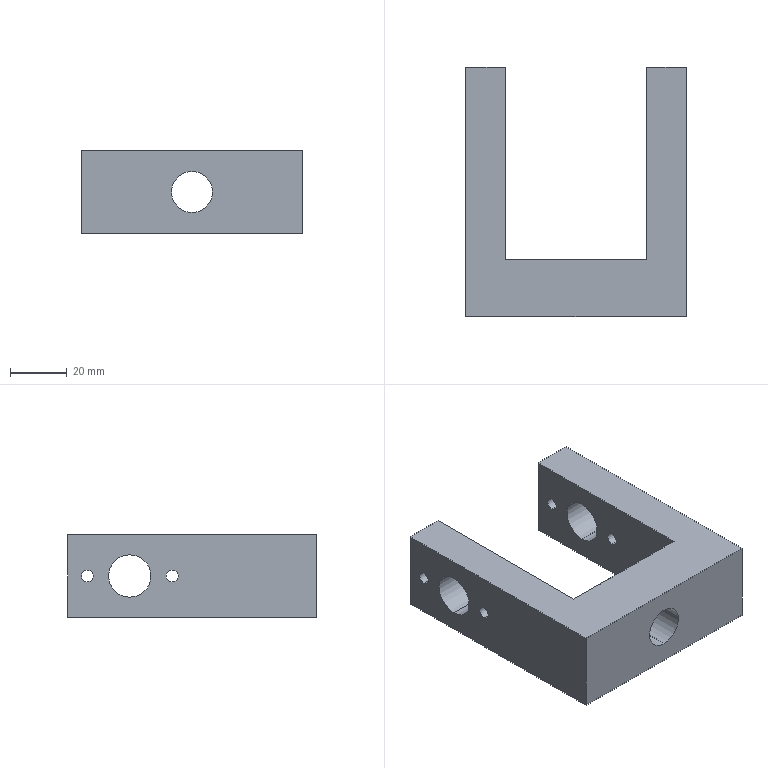Part | STEP file | PN_0050 (connecting block) | 1 solid | 24 faces | box 78 x 88 x 29 mm | volume 91430 mm3 | cylinder 14 | plane 10 | commonest cylinder face diameters 4.2 x8 15 x4 14.5 x2